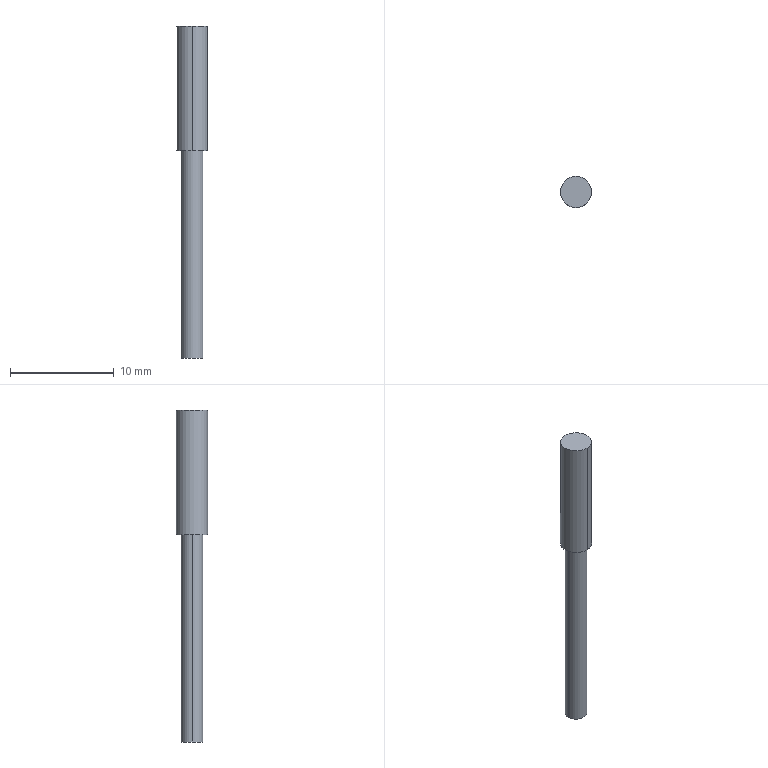Part | NX | 1 solid | 7 faces | box 3 x 3 x 32 mm | volume 154.095 mm3 | cylinder 4 | plane 3 | commonest cylinder face diameters 2.1 x2 3 x2
STEP:
#1=CARTESIAN_POINT('',(1.05,0.,0.));
#2=VERTEX_POINT('',#1);
#3=CARTESIAN_POINT('',(-1.05,0.,0.));
#4=VERTEX_POINT('',#3);
#5=CARTESIAN_POINT('',(0.,0.,0.));
#6=DIRECTION('',(0.,0.,1.));
#7=DIRECTION('',(-1.,0.,0.));
#8=AXIS2_PLACEMENT_3D('',#5,#6,#7);
#9=CIRCLE('',#8,1.05);
#10=EDGE_CURVE('',#2,#4,#9,.T.);
#11=ORIENTED_EDGE('',*,*,#10,.F.);
#12=CARTESIAN_POINT('',(0.,0.,0.));
#13=DIRECTION('',(0.,0.,1.));
#14=DIRECTION('',(-1.,0.,0.));
#15=AXIS2_PLACEMENT_3D('',#12,#13,#14);
#16=CIRCLE('',#15,1.05);
#17=EDGE_CURVE('',#4,#2,#16,.T.);
#18=ORIENTED_EDGE('',*,*,#17,.F.);
#19=EDGE_LOOP('',(#11,#18));
#20=FACE_BOUND('',#19,.T.);
#21=CARTESIAN_POINT('',(0.,0.,0.));
#22=DIRECTION('',(0.,0.,1.));
#23=DIRECTION('',(1.,0.,0.));
#24=AXIS2_PLACEMENT_3D('',#21,#22,#23);
#25=PLANE('',#24);
#26=ADVANCED_FACE('',(#20),#25,.F.);
#27=CARTESIAN_POINT('',(-1.05,0.,20.));
#28=VERTEX_POINT('',#27);
#29=CARTESIAN_POINT('',(1.05,0.,20.));
#30=VERTEX_POINT('',#29);
#31=CARTESIAN_POINT('',(0.,0.,20.));
#32=DIRECTION('',(0.,0.,-1.));
#33=DIRECTION('',(1.,0.,0.));
#34=AXIS2_PLACEMENT_3D('',#31,#32,#33);
#35=CIRCLE('',#34,1.05);
#36=EDGE_CURVE('',#28,#30,#35,.T.);
#37=ORIENTED_EDGE('',*,*,#36,.T.);
#38=CARTESIAN_POINT('',(1.05,0.,0.));
#39=DIRECTION('',(0.,0.,1.));
#40=VECTOR('',#39,1000.);
#41=LINE('',#38,#40);
#42=EDGE_CURVE('',#2,#30,#41,.T.);
#43=ORIENTED_EDGE('',*,*,#42,.F.);
#44=ORIENTED_EDGE('',*,*,#10,.T.);
#45=CARTESIAN_POINT('',(-1.05,0.,0.));
#46=DIRECTION('',(0.,0.,1.));
#47=VECTOR('',#46,1000.);
#48=LINE('',#45,#47);
#49=EDGE_CURVE('',#4,#28,#48,.T.);
#50=ORIENTED_EDGE('',*,*,#49,.T.);
#51=EDGE_LOOP('',(#37,#43,#44,#50));
#52=FACE_BOUND('',#51,.T.);
#53=CARTESIAN_POINT('',(0.,0.,0.));
#54=DIRECTION('',(0.,0.,1.));
#55=DIRECTION('',(1.,0.,0.));
#56=AXIS2_PLACEMENT_3D('',#53,#54,#55);
#57=CYLINDRICAL_SURFACE('',#56,1.05);
#58=ADVANCED_FACE('',(#52),#57,.T.);
#59=CARTESIAN_POINT('',(0.,1.5,20.));
#60=VERTEX_POINT('',#59);
#61=CARTESIAN_POINT('',(0.,-1.5,20.));
#62=VERTEX_POINT('',#61);
#63=CARTESIAN_POINT('',(0.,0.,20.));
#64=DIRECTION('',(0.,0.,1.));
#65=DIRECTION('',(0.,1.,0.));
#66=AXIS2_PLACEMENT_3D('',#63,#64,#65);
#67=CIRCLE('',#66,1.5);
#68=EDGE_CURVE('',#60,#62,#67,.T.);
#69=ORIENTED_EDGE('',*,*,#68,.F.);
#70=CARTESIAN_POINT('',(0.,0.,20.));
#71=DIRECTION('',(0.,0.,1.));
#72=DIRECTION('',(0.,1.,0.));
#73=AXIS2_PLACEMENT_3D('',#70,#71,#72);
#74=CIRCLE('',#73,1.5);
#75=EDGE_CURVE('',#62,#60,#74,.T.);
#76=ORIENTED_EDGE('',*,*,#75,.F.);
#77=EDGE_LOOP('',(#69,#76));
#78=FACE_BOUND('',#77,.T.);
#79=ORIENTED_EDGE('',*,*,#36,.F.);
#80=CARTESIAN_POINT('',(0.,0.,20.));
#81=DIRECTION('',(0.,0.,-1.));
#82=DIRECTION('',(1.,0.,0.));
#83=AXIS2_PLACEMENT_3D('',#80,#81,#82);
#84=CIRCLE('',#83,1.05);
#85=EDGE_CURVE('',#30,#28,#84,.T.);
#86=ORIENTED_EDGE('',*,*,#85,.F.);
#87=EDGE_LOOP('',(#79,#86));
#88=FACE_BOUND('',#87,.T.);
#89=CARTESIAN_POINT('',(0.,0.,20.));
#90=DIRECTION('',(0.,0.,1.));
#91=DIRECTION('',(1.,0.,0.));
#92=AXIS2_PLACEMENT_3D('',#89,#90,#91);
#93=PLANE('',#92);
#94=ADVANCED_FACE('',(#78,#88),#93,.F.);
#95=CARTESIAN_POINT('',(0.,1.5,32.));
#96=VERTEX_POINT('',#95);
#97=CARTESIAN_POINT('',(0.,-1.5,32.));
#98=VERTEX_POINT('',#97);
#99=CARTESIAN_POINT('',(0.,0.,32.));
#100=DIRECTION('',(0.,0.,-1.));
#101=DIRECTION('',(0.,-1.,0.));
#102=AXIS2_PLACEMENT_3D('',#99,#100,#101);
#103=CIRCLE('',#102,1.5);
#104=EDGE_CURVE('',#96,#98,#103,.T.);
#105=ORIENTED_EDGE('',*,*,#104,.T.);
#106=CARTESIAN_POINT('',(0.,-1.5,20.));
#107=DIRECTION('',(0.,0.,1.));
#108=VECTOR('',#107,1000.);
#109=LINE('',#106,#108);
#110=EDGE_CURVE('',#98,#62,#109,.F.);
#111=ORIENTED_EDGE('',*,*,#110,.T.);
#112=ORIENTED_EDGE('',*,*,#75,.T.);
#113=CARTESIAN_POINT('',(0.,1.5,20.));
#114=DIRECTION('',(0.,0.,1.));
#115=VECTOR('',#114,1000.);
#116=LINE('',#113,#115);
#117=EDGE_CURVE('',#96,#60,#116,.F.);
#118=ORIENTED_EDGE('',*,*,#117,.F.);
#119=EDGE_LOOP('',(#105,#111,#112,#118));
#120=FACE_BOUND('',#119,.T.);
#121=CARTESIAN_POINT('',(0.,0.,20.));
#122=DIRECTION('',(0.,0.,1.));
#123=DIRECTION('',(0.,-1.,0.));
#124=AXIS2_PLACEMENT_3D('',#121,#122,#123);
#125=CYLINDRICAL_SURFACE('',#124,1.5);
#126=ADVANCED_FACE('',(#120),#125,.T.);
#127=ORIENTED_EDGE('',*,*,#104,.F.);
#128=CARTESIAN_POINT('',(0.,0.,32.));
#129=DIRECTION('',(0.,0.,-1.));
#130=DIRECTION('',(0.,-1.,0.));
#131=AXIS2_PLACEMENT_3D('',#128,#129,#130);
#132=CIRCLE('',#131,1.5);
#133=EDGE_CURVE('',#98,#96,#132,.T.);
#134=ORIENTED_EDGE('',*,*,#133,.F.);
#135=EDGE_LOOP('',(#127,#134));
#136=FACE_BOUND('',#135,.T.);
#137=CARTESIAN_POINT('',(0.,0.,32.));
#138=DIRECTION('',(0.,0.,1.));
#139=DIRECTION('',(1.,0.,0.));
#140=AXIS2_PLACEMENT_3D('',#137,#138,#139);
#141=PLANE('',#140);
#142=ADVANCED_FACE('',(#136),#141,.T.);
#143=ORIENTED_EDGE('',*,*,#68,.T.);
#144=ORIENTED_EDGE('',*,*,#110,.F.);
#145=ORIENTED_EDGE('',*,*,#133,.T.);
#146=ORIENTED_EDGE('',*,*,#117,.T.);
#147=EDGE_LOOP('',(#143,#144,#145,#146));
#148=FACE_BOUND('',#147,.T.);
#149=CARTESIAN_POINT('',(0.,0.,20.));
#150=DIRECTION('',(0.,0.,1.));
#151=DIRECTION('',(0.,-1.,0.));
#152=AXIS2_PLACEMENT_3D('',#149,#150,#151);
#153=CYLINDRICAL_SURFACE('',#152,1.5);
#154=ADVANCED_FACE('',(#148),#153,.T.);
#155=ORIENTED_EDGE('',*,*,#42,.T.);
#156=ORIENTED_EDGE('',*,*,#85,.T.);
#157=ORIENTED_EDGE('',*,*,#49,.F.);
#158=ORIENTED_EDGE('',*,*,#17,.T.);
#159=EDGE_LOOP('',(#155,#156,#157,#158));
#160=FACE_BOUND('',#159,.T.);
#161=CARTESIAN_POINT('',(0.,0.,0.));
#162=DIRECTION('',(0.,0.,1.));
#163=DIRECTION('',(1.,0.,0.));
#164=AXIS2_PLACEMENT_3D('',#161,#162,#163);
#165=CYLINDRICAL_SURFACE('',#164,1.05);
#166=ADVANCED_FACE('',(#160),#165,.T.);
#167=CLOSED_SHELL('',(#26,#58,#94,#126,#142,#154,#166));
#168=MANIFOLD_SOLID_BREP('',#167);
#169=(LENGTH_UNIT()NAMED_UNIT(*)SI_UNIT(.MILLI.,.METRE.));
#170=UNCERTAINTY_MEASURE_WITH_UNIT(LENGTH_MEASURE(0.00001),#169,'','');
#171=(NAMED_UNIT(*)PLANE_ANGLE_UNIT()SI_UNIT($,.RADIAN.));
#172=(NAMED_UNIT(*)SI_UNIT($,.STERADIAN.)SOLID_ANGLE_UNIT());
#173=(GEOMETRIC_REPRESENTATION_CONTEXT(3)GLOBAL_UNCERTAINTY_ASSIGNED_CONTEXT((#170))GLOBAL_UNIT_ASSIGNED_CONTEXT((#169,#171,#172))REPRESENTATION_CONTEXT('',''));
#174=ADVANCED_BREP_SHAPE_REPRESENTATION('',(#168),#173);